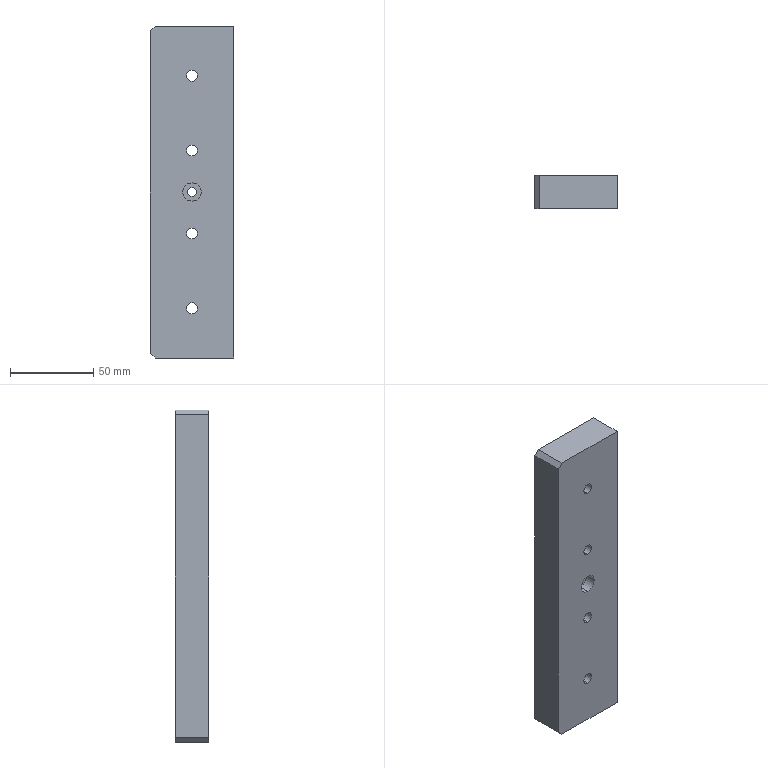Part | SolidWorks | features HoleWzd 3, Chamfer 1, Extrusion 1 | 1 solid | 45 faces | box 50 x 20 x 200 mm | volume 193251 mm3 | cylinder 26 | plane 13 | cone 6 | commonest cylinder face diameters 11 x10 5.2 x8 6.6 x8
STEP:
#1=CARTESIAN_POINT('',(0.,-3.6,5.5));
#2=VERTEX_POINT('',#1);
#3=CARTESIAN_POINT('',(0.,-3.6,-5.5));
#4=VERTEX_POINT('',#3);
#5=CARTESIAN_POINT('',(0.,-3.6,0.));
#6=DIRECTION('',(0.,-1.,0.));
#7=DIRECTION('',(0.,0.,-1.));
#8=AXIS2_PLACEMENT_3D('',#5,#6,#7);
#9=CIRCLE('',#8,5.5);
#10=EDGE_CURVE('',#2,#4,#9,.T.);
#11=ORIENTED_EDGE('',*,*,#10,.F.);
#12=CARTESIAN_POINT('',(0.,-10.,5.5));
#13=VERTEX_POINT('',#12);
#14=CARTESIAN_POINT('',(0.,-10.,5.5));
#15=DIRECTION('',(0.,-1.,0.));
#16=VECTOR('',#15,1000.);
#17=LINE('',#14,#16);
#18=EDGE_CURVE('',#2,#13,#17,.T.);
#19=ORIENTED_EDGE('',*,*,#18,.T.);
#20=CARTESIAN_POINT('',(0.,-10.,-5.5));
#21=VERTEX_POINT('',#20);
#22=CARTESIAN_POINT('',(0.,-10.,0.));
#23=DIRECTION('',(0.,-1.,0.));
#24=DIRECTION('',(0.,0.,-1.));
#25=AXIS2_PLACEMENT_3D('',#22,#23,#24);
#26=CIRCLE('',#25,5.5);
#27=EDGE_CURVE('',#13,#21,#26,.T.);
#28=ORIENTED_EDGE('',*,*,#27,.T.);
#29=CARTESIAN_POINT('',(0.,-10.,-5.5));
#30=DIRECTION('',(0.,-1.,0.));
#31=VECTOR('',#30,1000.);
#32=LINE('',#29,#31);
#33=EDGE_CURVE('',#4,#21,#32,.T.);
#34=ORIENTED_EDGE('',*,*,#33,.F.);
#35=EDGE_LOOP('',(#11,#19,#28,#34));
#36=FACE_OUTER_BOUND('',#35,.T.);
#37=CARTESIAN_POINT('',(0.,-10.,0.));
#38=DIRECTION('',(0.,-1.,0.));
#39=DIRECTION('',(0.,0.,-1.));
#40=AXIS2_PLACEMENT_3D('',#37,#38,#39);
#41=CYLINDRICAL_SURFACE('',#40,5.5);
#42=ADVANCED_FACE('',(#36),#41,.F.);
#43=CARTESIAN_POINT('',(0.,10.,2.6));
#44=VERTEX_POINT('',#43);
#45=CARTESIAN_POINT('',(0.,10.,-2.6));
#46=VERTEX_POINT('',#45);
#47=CARTESIAN_POINT('',(0.,10.,0.));
#48=DIRECTION('',(0.,-1.,0.));
#49=DIRECTION('',(0.,0.,-1.));
#50=AXIS2_PLACEMENT_3D('',#47,#48,#49);
#51=CIRCLE('',#50,2.6);
#52=EDGE_CURVE('',#44,#46,#51,.T.);
#53=ORIENTED_EDGE('',*,*,#52,.F.);
#54=CARTESIAN_POINT('',(0.,-3.6,2.6));
#55=VERTEX_POINT('',#54);
#56=CARTESIAN_POINT('',(0.,-10.,2.6));
#57=DIRECTION('',(0.,-1.,0.));
#58=VECTOR('',#57,1000.);
#59=LINE('',#56,#58);
#60=EDGE_CURVE('',#44,#55,#59,.T.);
#61=ORIENTED_EDGE('',*,*,#60,.T.);
#62=CARTESIAN_POINT('',(0.,-3.6,-2.6));
#63=VERTEX_POINT('',#62);
#64=CARTESIAN_POINT('',(0.,-3.6,0.));
#65=DIRECTION('',(0.,-1.,0.));
#66=DIRECTION('',(0.,0.,-1.));
#67=AXIS2_PLACEMENT_3D('',#64,#65,#66);
#68=CIRCLE('',#67,2.6);
#69=EDGE_CURVE('',#55,#63,#68,.T.);
#70=ORIENTED_EDGE('',*,*,#69,.T.);
#71=CARTESIAN_POINT('',(0.,-10.,-2.6));
#72=DIRECTION('',(0.,-1.,0.));
#73=VECTOR('',#72,1000.);
#74=LINE('',#71,#73);
#75=EDGE_CURVE('',#46,#63,#74,.T.);
#76=ORIENTED_EDGE('',*,*,#75,.F.);
#77=EDGE_LOOP('',(#53,#61,#70,#76));
#78=FACE_OUTER_BOUND('',#77,.T.);
#79=CARTESIAN_POINT('',(0.,-10.,0.));
#80=DIRECTION('',(0.,-1.,0.));
#81=DIRECTION('',(0.,0.,-1.));
#82=AXIS2_PLACEMENT_3D('',#79,#80,#81);
#83=CYLINDRICAL_SURFACE('',#82,2.6);
#84=ADVANCED_FACE('',(#78),#83,.F.);
#85=CARTESIAN_POINT('',(10.,0.,87.6));
#86=VERTEX_POINT('',#85);
#87=CARTESIAN_POINT('',(10.,0.,82.4));
#88=VERTEX_POINT('',#87);
#89=CARTESIAN_POINT('',(10.,0.,85.));
#90=DIRECTION('',(1.,0.,0.));
#91=DIRECTION('',(0.,0.,-1.));
#92=AXIS2_PLACEMENT_3D('',#89,#90,#91);
#93=CIRCLE('',#92,2.6);
#94=EDGE_CURVE('',#86,#88,#93,.T.);
#95=ORIENTED_EDGE('',*,*,#94,.F.);
#96=CARTESIAN_POINT('',(25.,0.,87.6));
#97=VERTEX_POINT('',#96);
#98=CARTESIAN_POINT('',(25.,0.,87.6));
#99=DIRECTION('',(1.,0.,0.));
#100=VECTOR('',#99,1000.);
#101=LINE('',#98,#100);
#102=EDGE_CURVE('',#86,#97,#101,.T.);
#103=ORIENTED_EDGE('',*,*,#102,.T.);
#104=CARTESIAN_POINT('',(25.,0.,82.4));
#105=VERTEX_POINT('',#104);
#106=CARTESIAN_POINT('',(25.,0.,85.));
#107=DIRECTION('',(1.,0.,0.));
#108=DIRECTION('',(0.,0.,-1.));
#109=AXIS2_PLACEMENT_3D('',#106,#107,#108);
#110=CIRCLE('',#109,2.6);
#111=EDGE_CURVE('',#97,#105,#110,.T.);
#112=ORIENTED_EDGE('',*,*,#111,.T.);
#113=CARTESIAN_POINT('',(25.,0.,82.4));
#114=DIRECTION('',(1.,0.,0.));
#115=VECTOR('',#114,1000.);
#116=LINE('',#113,#115);
#117=EDGE_CURVE('',#88,#105,#116,.T.);
#118=ORIENTED_EDGE('',*,*,#117,.F.);
#119=EDGE_LOOP('',(#95,#103,#112,#118));
#120=FACE_OUTER_BOUND('',#119,.T.);
#121=CARTESIAN_POINT('',(25.,0.,85.));
#122=DIRECTION('',(1.,0.,0.));
#123=DIRECTION('',(0.,0.,-1.));
#124=AXIS2_PLACEMENT_3D('',#121,#122,#123);
#125=CYLINDRICAL_SURFACE('',#124,2.6);
#126=ADVANCED_FACE('',(#120),#125,.F.);
#127=CARTESIAN_POINT('',(8.438,0.,85.));
#128=VERTEX_POINT('',#127);
#129=CARTESIAN_POINT('',(10.,0.,82.4));
#130=DIRECTION('',(0.515,0.,-0.8572));
#131=VECTOR('',#130,1000.);
#132=LINE('',#129,#131);
#133=EDGE_CURVE('',#128,#88,#132,.T.);
#134=ORIENTED_EDGE('',*,*,#133,.F.);
#135=CARTESIAN_POINT('',(10.,0.,87.6));
#136=DIRECTION('',(0.515,0.,0.8572));
#137=VECTOR('',#136,1000.);
#138=LINE('',#135,#137);
#139=EDGE_CURVE('',#128,#86,#138,.T.);
#140=ORIENTED_EDGE('',*,*,#139,.T.);
#141=ORIENTED_EDGE('',*,*,#94,.T.);
#142=EDGE_LOOP('',(#134,#140,#141));
#143=FACE_OUTER_BOUND('',#142,.T.);
#144=CARTESIAN_POINT('',(10.,0.,85.));
#145=DIRECTION('',(1.,0.,0.));
#146=DIRECTION('',(0.,0.,-1.));
#147=AXIS2_PLACEMENT_3D('',#144,#145,#146);
#148=CONICAL_SURFACE('',#147,2.6,1.03);
#149=ADVANCED_FACE('',(#143),#148,.F.);
#150=CARTESIAN_POINT('',(10.,0.,2.6));
#151=VERTEX_POINT('',#150);
#152=CARTESIAN_POINT('',(10.,0.,-2.6));
#153=VERTEX_POINT('',#152);
#154=CARTESIAN_POINT('',(10.,0.,0.));
#155=DIRECTION('',(1.,0.,0.));
#156=DIRECTION('',(0.,0.,-1.));
#157=AXIS2_PLACEMENT_3D('',#154,#155,#156);
#158=CIRCLE('',#157,2.6);
#159=EDGE_CURVE('',#151,#153,#158,.T.);
#160=ORIENTED_EDGE('',*,*,#159,.F.);
#161=CARTESIAN_POINT('',(25.,0.,2.6));
#162=VERTEX_POINT('',#161);
#163=CARTESIAN_POINT('',(25.,0.,2.6));
#164=DIRECTION('',(1.,0.,0.));
#165=VECTOR('',#164,1000.);
#166=LINE('',#163,#165);
#167=EDGE_CURVE('',#151,#162,#166,.T.);
#168=ORIENTED_EDGE('',*,*,#167,.T.);
#169=CARTESIAN_POINT('',(25.,0.,-2.6));
#170=VERTEX_POINT('',#169);
#171=CARTESIAN_POINT('',(25.,0.,0.));
#172=DIRECTION('',(1.,0.,0.));
#173=DIRECTION('',(0.,0.,-1.));
#174=AXIS2_PLACEMENT_3D('',#171,#172,#173);
#175=CIRCLE('',#174,2.6);
#176=EDGE_CURVE('',#162,#170,#175,.T.);
#177=ORIENTED_EDGE('',*,*,#176,.T.);
#178=CARTESIAN_POINT('',(25.,0.,-2.6));
#179=DIRECTION('',(1.,0.,0.));
#180=VECTOR('',#179,1000.);
#181=LINE('',#178,#180);
#182=EDGE_CURVE('',#153,#170,#181,.T.);
#183=ORIENTED_EDGE('',*,*,#182,.F.);
#184=EDGE_LOOP('',(#160,#168,#177,#183));
#185=FACE_OUTER_BOUND('',#184,.T.);
#186=CARTESIAN_POINT('',(25.,0.,0.));
#187=DIRECTION('',(1.,0.,0.));
#188=DIRECTION('',(0.,0.,-1.));
#189=AXIS2_PLACEMENT_3D('',#186,#187,#188);
#190=CYLINDRICAL_SURFACE('',#189,2.6);
#191=ADVANCED_FACE('',(#185),#190,.F.);
#192=CARTESIAN_POINT('',(8.438,0.,0.));
#193=VERTEX_POINT('',#192);
#194=CARTESIAN_POINT('',(10.,0.,-2.6));
#195=DIRECTION('',(0.515,0.,-0.8572));
#196=VECTOR('',#195,1000.);
#197=LINE('',#194,#196);
#198=EDGE_CURVE('',#193,#153,#197,.T.);
#199=ORIENTED_EDGE('',*,*,#198,.F.);
#200=CARTESIAN_POINT('',(10.,0.,2.6));
#201=DIRECTION('',(0.515,0.,0.8572));
#202=VECTOR('',#201,1000.);
#203=LINE('',#200,#202);
#204=EDGE_CURVE('',#193,#151,#203,.T.);
#205=ORIENTED_EDGE('',*,*,#204,.T.);
#206=ORIENTED_EDGE('',*,*,#159,.T.);
#207=EDGE_LOOP('',(#199,#205,#206));
#208=FACE_OUTER_BOUND('',#207,.T.);
#209=CARTESIAN_POINT('',(10.,0.,0.));
#210=DIRECTION('',(1.,0.,0.));
#211=DIRECTION('',(0.,0.,-1.));
#212=AXIS2_PLACEMENT_3D('',#209,#210,#211);
#213=CONICAL_SURFACE('',#212,2.6,1.03);
#214=ADVANCED_FACE('',(#208),#213,.F.);
#215=CARTESIAN_POINT('',(10.,0.,-82.4));
#216=VERTEX_POINT('',#215);
#217=CARTESIAN_POINT('',(10.,0.,-87.6));
#218=VERTEX_POINT('',#217);
#219=CARTESIAN_POINT('',(10.,0.,-85.));
#220=DIRECTION('',(1.,0.,0.));
#221=DIRECTION('',(0.,0.,-1.));
#222=AXIS2_PLACEMENT_3D('',#219,#220,#221);
#223=CIRCLE('',#222,2.6);
#224=EDGE_CURVE('',#216,#218,#223,.T.);
#225=ORIENTED_EDGE('',*,*,#224,.F.);
#226=CARTESIAN_POINT('',(25.,0.,-82.4));
#227=VERTEX_POINT('',#226);
#228=CARTESIAN_POINT('',(25.,0.,-82.4));
#229=DIRECTION('',(1.,0.,0.));
#230=VECTOR('',#229,1000.);
#231=LINE('',#228,#230);
#232=EDGE_CURVE('',#216,#227,#231,.T.);
#233=ORIENTED_EDGE('',*,*,#232,.T.);
#234=CARTESIAN_POINT('',(25.,0.,-87.6));
#235=VERTEX_POINT('',#234);
#236=CARTESIAN_POINT('',(25.,0.,-85.));
#237=DIRECTION('',(1.,0.,0.));
#238=DIRECTION('',(0.,0.,-1.));
#239=AXIS2_PLACEMENT_3D('',#236,#237,#238);
#240=CIRCLE('',#239,2.6);
#241=EDGE_CURVE('',#227,#235,#240,.T.);
#242=ORIENTED_EDGE('',*,*,#241,.T.);
#243=CARTESIAN_POINT('',(25.,0.,-87.6));
#244=DIRECTION('',(1.,0.,0.));
#245=VECTOR('',#244,1000.);
#246=LINE('',#243,#245);
#247=EDGE_CURVE('',#218,#235,#246,.T.);
#248=ORIENTED_EDGE('',*,*,#247,.F.);
#249=EDGE_LOOP('',(#225,#233,#242,#248));
#250=FACE_OUTER_BOUND('',#249,.T.);
#251=CARTESIAN_POINT('',(25.,0.,-85.));
#252=DIRECTION('',(1.,0.,0.));
#253=DIRECTION('',(0.,0.,-1.));
#254=AXIS2_PLACEMENT_3D('',#251,#252,#253);
#255=CYLINDRICAL_SURFACE('',#254,2.6);
#256=ADVANCED_FACE('',(#250),#255,.F.);
#257=CARTESIAN_POINT('',(8.438,0.,-85.));
#258=VERTEX_POINT('',#257);
#259=CARTESIAN_POINT('',(10.,0.,-87.6));
#260=DIRECTION('',(0.515,0.,-0.8572));
#261=VECTOR('',#260,1000.);
#262=LINE('',#259,#261);
#263=EDGE_CURVE('',#258,#218,#262,.T.);
#264=ORIENTED_EDGE('',*,*,#263,.F.);
#265=CARTESIAN_POINT('',(10.,0.,-82.4));
#266=DIRECTION('',(0.515,0.,0.8572));
#267=VECTOR('',#266,1000.);
#268=LINE('',#265,#267);
#269=EDGE_CURVE('',#258,#216,#268,.T.);
#270=ORIENTED_EDGE('',*,*,#269,.T.);
#271=ORIENTED_EDGE('',*,*,#224,.T.);
#272=EDGE_LOOP('',(#264,#270,#271));
#273=FACE_OUTER_BOUND('',#272,.T.);
#274=CARTESIAN_POINT('',(10.,0.,-85.));
#275=DIRECTION('',(1.,0.,0.));
#276=DIRECTION('',(0.,0.,-1.));
#277=AXIS2_PLACEMENT_3D('',#274,#275,#276);
#278=CONICAL_SURFACE('',#277,2.6,1.03);
#279=ADVANCED_FACE('',(#273),#278,.F.);
#280=CARTESIAN_POINT('',(0.,2.,-75.5));
#281=VERTEX_POINT('',#280);
#282=CARTESIAN_POINT('',(0.,2.,-64.5));
#283=VERTEX_POINT('',#282);
#284=CARTESIAN_POINT('',(0.,2.,-70.));
#285=DIRECTION('',(0.,1.,0.));
#286=DIRECTION('',(0.,0.,1.));
#287=AXIS2_PLACEMENT_3D('',#284,#285,#286);
#288=CIRCLE('',#287,5.5);
#289=EDGE_CURVE('',#281,#283,#288,.T.);
#290=ORIENTED_EDGE('',*,*,#289,.F.);
#291=CARTESIAN_POINT('',(0.,10.,-75.5));
#292=VERTEX_POINT('',#291);
#293=CARTESIAN_POINT('',(0.,10.,-75.5));
#294=DIRECTION('',(0.,1.,0.));
#295=VECTOR('',#294,1000.);
#296=LINE('',#293,#295);
#297=EDGE_CURVE('',#281,#292,#296,.T.);
#298=ORIENTED_EDGE('',*,*,#297,.T.);
#299=CARTESIAN_POINT('',(0.,10.,-64.5));
#300=VERTEX_POINT('',#299);
#301=CARTESIAN_POINT('',(0.,10.,-70.));
#302=DIRECTION('',(0.,1.,0.));
#303=DIRECTION('',(0.,0.,1.));
#304=AXIS2_PLACEMENT_3D('',#301,#302,#303);
#305=CIRCLE('',#304,5.5);
#306=EDGE_CURVE('',#292,#300,#305,.T.);
#307=ORIENTED_EDGE('',*,*,#306,.T.);
#308=CARTESIAN_POINT('',(0.,10.,-64.5));
#309=DIRECTION('',(0.,1.,0.));
#310=VECTOR('',#309,1000.);
#311=LINE('',#308,#310);
#312=EDGE_CURVE('',#283,#300,#311,.T.);
#313=ORIENTED_EDGE('',*,*,#312,.F.);
#314=EDGE_LOOP('',(#290,#298,#307,#313));
#315=FACE_OUTER_BOUND('',#314,.T.);
#316=CARTESIAN_POINT('',(0.,10.,-70.));
#317=DIRECTION('',(0.,1.,0.));
#318=DIRECTION('',(0.,0.,1.));
#319=AXIS2_PLACEMENT_3D('',#316,#317,#318);
#320=CYLINDRICAL_SURFACE('',#319,5.5);
#321=ADVANCED_FACE('',(#315),#320,.F.);
#322=CARTESIAN_POINT('',(0.,-10.,-73.3));
#323=VERTEX_POINT('',#322);
#324=CARTESIAN_POINT('',(0.,-10.,-66.7));
#325=VERTEX_POINT('',#324);
#326=CARTESIAN_POINT('',(0.,-10.,-70.));
#327=DIRECTION('',(0.,1.,0.));
#328=DIRECTION('',(0.,0.,1.));
#329=AXIS2_PLACEMENT_3D('',#326,#327,#328);
#330=CIRCLE('',#329,3.3);
#331=EDGE_CURVE('',#323,#325,#330,.T.);
#332=ORIENTED_EDGE('',*,*,#331,.F.);
#333=CARTESIAN_POINT('',(0.,2.,-73.3));
#334=VERTEX_POINT('',#333);
#335=CARTESIAN_POINT('',(0.,10.,-73.3));
#336=DIRECTION('',(0.,1.,0.));
#337=VECTOR('',#336,1000.);
#338=LINE('',#335,#337);
#339=EDGE_CURVE('',#323,#334,#338,.T.);
#340=ORIENTED_EDGE('',*,*,#339,.T.);
#341=CARTESIAN_POINT('',(0.,2.,-66.7));
#342=VERTEX_POINT('',#341);
#343=CARTESIAN_POINT('',(0.,2.,-70.));
#344=DIRECTION('',(0.,1.,0.));
#345=DIRECTION('',(0.,0.,1.));
#346=AXIS2_PLACEMENT_3D('',#343,#344,#345);
#347=CIRCLE('',#346,3.3);
#348=EDGE_CURVE('',#334,#342,#347,.T.);
#349=ORIENTED_EDGE('',*,*,#348,.T.);
#350=CARTESIAN_POINT('',(0.,10.,-66.7));
#351=DIRECTION('',(0.,1.,0.));
#352=VECTOR('',#351,1000.);
#353=LINE('',#350,#352);
#354=EDGE_CURVE('',#325,#342,#353,.T.);
#355=ORIENTED_EDGE('',*,*,#354,.F.);
#356=EDGE_LOOP('',(#332,#340,#349,#355));
#357=FACE_OUTER_BOUND('',#356,.T.);
#358=CARTESIAN_POINT('',(0.,10.,-70.));
#359=DIRECTION('',(0.,1.,0.));
#360=DIRECTION('',(0.,0.,1.));
#361=AXIS2_PLACEMENT_3D('',#358,#359,#360);
#362=CYLINDRICAL_SURFACE('',#361,3.3);
#363=ADVANCED_FACE('',(#357),#362,.F.);
#364=CARTESIAN_POINT('',(0.,2.,64.5));
#365=VERTEX_POINT('',#364);
#366=CARTESIAN_POINT('',(0.,2.,75.5));
#367=VERTEX_POINT('',#366);
#368=CARTESIAN_POINT('',(0.,2.,70.));
#369=DIRECTION('',(0.,1.,0.));
#370=DIRECTION('',(0.,0.,1.));
#371=AXIS2_PLACEMENT_3D('',#368,#369,#370);
#372=CIRCLE('',#371,5.5);
#373=EDGE_CURVE('',#365,#367,#372,.T.);
#374=ORIENTED_EDGE('',*,*,#373,.F.);
#375=CARTESIAN_POINT('',(0.,10.,64.5));
#376=VERTEX_POINT('',#375);
#377=CARTESIAN_POINT('',(0.,10.,64.5));
#378=DIRECTION('',(0.,1.,0.));
#379=VECTOR('',#378,1000.);
#380=LINE('',#377,#379);
#381=EDGE_CURVE('',#365,#376,#380,.T.);
#382=ORIENTED_EDGE('',*,*,#381,.T.);
#383=CARTESIAN_POINT('',(0.,10.,75.5));
#384=VERTEX_POINT('',#383);
#385=CARTESIAN_POINT('',(0.,10.,70.));
#386=DIRECTION('',(0.,1.,0.));
#387=DIRECTION('',(0.,0.,1.));
#388=AXIS2_PLACEMENT_3D('',#385,#386,#387);
#389=CIRCLE('',#388,5.5);
#390=EDGE_CURVE('',#376,#384,#389,.T.);
#391=ORIENTED_EDGE('',*,*,#390,.T.);
#392=CARTESIAN_POINT('',(0.,10.,75.5));
#393=DIRECTION('',(0.,1.,0.));
#394=VECTOR('',#393,1000.);
#395=LINE('',#392,#394);
#396=EDGE_CURVE('',#367,#384,#395,.T.);
#397=ORIENTED_EDGE('',*,*,#396,.F.);
#398=EDGE_LOOP('',(#374,#382,#391,#397));
#399=FACE_OUTER_BOUND('',#398,.T.);
#400=CARTESIAN_POINT('',(0.,10.,70.));
#401=DIRECTION('',(0.,1.,0.));
#402=DIRECTION('',(0.,0.,1.));
#403=AXIS2_PLACEMENT_3D('',#400,#401,#402);
#404=CYLINDRICAL_SURFACE('',#403,5.5);
#405=ADVANCED_FACE('',(#399),#404,.F.);
#406=CARTESIAN_POINT('',(0.,-10.,66.7));
#407=VERTEX_POINT('',#406);
#408=CARTESIAN_POINT('',(0.,-10.,73.3));
#409=VERTEX_POINT('',#408);
#410=CARTESIAN_POINT('',(0.,-10.,70.));
#411=DIRECTION('',(0.,1.,0.));
#412=DIRECTION('',(0.,0.,1.));
#413=AXIS2_PLACEMENT_3D('',#410,#411,#412);
#414=CIRCLE('',#413,3.3);
#415=EDGE_CURVE('',#407,#409,#414,.T.);
#416=ORIENTED_EDGE('',*,*,#415,.F.);
#417=CARTESIAN_POINT('',(0.,2.,66.7));
#418=VERTEX_POINT('',#417);
#419=CARTESIAN_POINT('',(0.,10.,66.7));
#420=DIRECTION('',(0.,1.,0.));
#421=VECTOR('',#420,1000.);
#422=LINE('',#419,#421);
#423=EDGE_CURVE('',#407,#418,#422,.T.);
#424=ORIENTED_EDGE('',*,*,#423,.T.);
#425=CARTESIAN_POINT('',(0.,2.,73.3));
#426=VERTEX_POINT('',#425);
#427=CARTESIAN_POINT('',(0.,2.,70.));
#428=DIRECTION('',(0.,1.,0.));
#429=DIRECTION('',(0.,0.,1.));
#430=AXIS2_PLACEMENT_3D('',#427,#428,#429);
#431=CIRCLE('',#430,3.3);
#432=EDGE_CURVE('',#418,#426,#431,.T.);
#433=ORIENTED_EDGE('',*,*,#432,.T.);
#434=CARTESIAN_POINT('',(0.,10.,73.3));
#435=DIRECTION('',(0.,1.,0.));
#436=VECTOR('',#435,1000.);
#437=LINE('',#434,#436);
#438=EDGE_CURVE('',#409,#426,#437,.T.);
#439=ORIENTED_EDGE('',*,*,#438,.F.);
#440=EDGE_LOOP('',(#416,#424,#433,#439));
#441=FACE_OUTER_BOUND('',#440,.T.);
#442=CARTESIAN_POINT('',(0.,10.,70.));
#443=DIRECTION('',(0.,1.,0.));
#444=DIRECTION('',(0.,0.,1.));
#445=AXIS2_PLACEMENT_3D('',#442,#443,#444);
#446=CYLINDRICAL_SURFACE('',#445,3.3);
#447=ADVANCED_FACE('',(#441),#446,.F.);
#448=CARTESIAN_POINT('',(0.,2.,-30.5));
#449=VERTEX_POINT('',#448);
#450=CARTESIAN_POINT('',(0.,2.,-19.5));
#451=VERTEX_POINT('',#450);
#452=CARTESIAN_POINT('',(0.,2.,-25.));
#453=DIRECTION('',(0.,1.,0.));
#454=DIRECTION('',(0.,0.,1.));
#455=AXIS2_PLACEMENT_3D('',#452,#453,#454);
#456=CIRCLE('',#455,5.5);
#457=EDGE_CURVE('',#449,#451,#456,.T.);
#458=ORIENTED_EDGE('',*,*,#457,.F.);
#459=CARTESIAN_POINT('',(0.,10.,-30.5));
#460=VERTEX_POINT('',#459);
#461=CARTESIAN_POINT('',(0.,10.,-30.5));
#462=DIRECTION('',(0.,1.,0.));
#463=VECTOR('',#462,1000.);
#464=LINE('',#461,#463);
#465=EDGE_CURVE('',#449,#460,#464,.T.);
#466=ORIENTED_EDGE('',*,*,#465,.T.);
#467=CARTESIAN_POINT('',(0.,10.,-19.5));
#468=VERTEX_POINT('',#467);
#469=CARTESIAN_POINT('',(0.,10.,-25.));
#470=DIRECTION('',(0.,1.,0.));
#471=DIRECTION('',(0.,0.,1.));
#472=AXIS2_PLACEMENT_3D('',#469,#470,#471);
#473=CIRCLE('',#472,5.5);
#474=EDGE_CURVE('',#460,#468,#473,.T.);
#475=ORIENTED_EDGE('',*,*,#474,.T.);
#476=CARTESIAN_POINT('',(0.,10.,-19.5));
#477=DIRECTION('',(0.,1.,0.));
#478=VECTOR('',#477,1000.);
#479=LINE('',#476,#478);
#480=EDGE_CURVE('',#451,#468,#479,.T.);
#481=ORIENTED_EDGE('',*,*,#480,.F.);
#482=EDGE_LOOP('',(#458,#466,#475,#481));
#483=FACE_OUTER_BOUND('',#482,.T.);
#484=CARTESIAN_POINT('',(0.,10.,-25.));
#485=DIRECTION('',(0.,1.,0.));
#486=DIRECTION('',(0.,0.,1.));
#487=AXIS2_PLACEMENT_3D('',#484,#485,#486);
#488=CYLINDRICAL_SURFACE('',#487,5.5);
#489=ADVANCED_FACE('',(#483),#488,.F.);
#490=CARTESIAN_POINT('',(0.,-10.,-28.3));
#491=VERTEX_POINT('',#490);
#492=CARTESIAN_POINT('',(0.,-10.,-21.7));
#493=VERTEX_POINT('',#492);
#494=CARTESIAN_POINT('',(0.,-10.,-25.));
#495=DIRECTION('',(0.,1.,0.));
#496=DIRECTION('',(0.,0.,1.));
#497=AXIS2_PLACEMENT_3D('',#494,#495,#496);
#498=CIRCLE('',#497,3.3);
#499=EDGE_CURVE('',#491,#493,#498,.T.);
#500=ORIENTED_EDGE('',*,*,#499,.F.);
#501=CARTESIAN_POINT('',(0.,2.,-28.3));
#502=VERTEX_POINT('',#501);
#503=CARTESIAN_POINT('',(0.,10.,-28.3));
#504=DIRECTION('',(0.,1.,0.));
#505=VECTOR('',#504,1000.);
#506=LINE('',#503,#505);
#507=EDGE_CURVE('',#491,#502,#506,.T.);
#508=ORIENTED_EDGE('',*,*,#507,.T.);
#509=CARTESIAN_POINT('',(0.,2.,-21.7));
#510=VERTEX_POINT('',#509);
#511=CARTESIAN_POINT('',(0.,2.,-25.));
#512=DIRECTION('',(0.,1.,0.));
#513=DIRECTION('',(0.,0.,1.));
#514=AXIS2_PLACEMENT_3D('',#511,#512,#513);
#515=CIRCLE('',#514,3.3);
#516=EDGE_CURVE('',#502,#510,#515,.T.);
#517=ORIENTED_EDGE('',*,*,#516,.T.);
#518=CARTESIAN_POINT('',(0.,10.,-21.7));
#519=DIRECTION('',(0.,1.,0.));
#520=VECTOR('',#519,1000.);
#521=LINE('',#518,#520);
#522=EDGE_CURVE('',#493,#510,#521,.T.);
#523=ORIENTED_EDGE('',*,*,#522,.F.);
#524=EDGE_LOOP('',(#500,#508,#517,#523));
#525=FACE_OUTER_BOUND('',#524,.T.);
#526=CARTESIAN_POINT('',(0.,10.,-25.));
#527=DIRECTION('',(0.,1.,0.));
#528=DIRECTION('',(0.,0.,1.));
#529=AXIS2_PLACEMENT_3D('',#526,#527,#528);
#530=CYLINDRICAL_SURFACE('',#529,3.3);
#531=ADVANCED_FACE('',(#525),#530,.F.);
#532=CARTESIAN_POINT('',(0.,2.,19.5));
#533=VERTEX_POINT('',#532);
#534=CARTESIAN_POINT('',(0.,2.,30.5));
#535=VERTEX_POINT('',#534);
#536=CARTESIAN_POINT('',(0.,2.,25.));
#537=DIRECTION('',(0.,1.,0.));
#538=DIRECTION('',(0.,0.,1.));
#539=AXIS2_PLACEMENT_3D('',#536,#537,#538);
#540=CIRCLE('',#539,5.5);
#541=EDGE_CURVE('',#533,#535,#540,.T.);
#542=ORIENTED_EDGE('',*,*,#541,.F.);
#543=CARTESIAN_POINT('',(0.,10.,19.5));
#544=VERTEX_POINT('',#543);
#545=CARTESIAN_POINT('',(0.,10.,19.5));
#546=DIRECTION('',(0.,1.,0.));
#547=VECTOR('',#546,1000.);
#548=LINE('',#545,#547);
#549=EDGE_CURVE('',#533,#544,#548,.T.);
#550=ORIENTED_EDGE('',*,*,#549,.T.);
#551=CARTESIAN_POINT('',(0.,10.,30.5));
#552=VERTEX_POINT('',#551);
#553=CARTESIAN_POINT('',(0.,10.,25.));
#554=DIRECTION('',(0.,1.,0.));
#555=DIRECTION('',(0.,0.,1.));
#556=AXIS2_PLACEMENT_3D('',#553,#554,#555);
#557=CIRCLE('',#556,5.5);
#558=EDGE_CURVE('',#544,#552,#557,.T.);
#559=ORIENTED_EDGE('',*,*,#558,.T.);
#560=CARTESIAN_POINT('',(0.,10.,30.5));
#561=DIRECTION('',(0.,1.,0.));
#562=VECTOR('',#561,1000.);
#563=LINE('',#560,#562);
#564=EDGE_CURVE('',#535,#552,#563,.T.);
#565=ORIENTED_EDGE('',*,*,#564,.F.);
#566=EDGE_LOOP('',(#542,#550,#559,#565));
#567=FACE_OUTER_BOUND('',#566,.T.);
#568=CARTESIAN_POINT('',(0.,10.,25.));
#569=DIRECTION('',(0.,1.,0.));
#570=DIRECTION('',(0.,0.,1.));
#571=AXIS2_PLACEMENT_3D('',#568,#569,#570);
#572=CYLINDRICAL_SURFACE('',#571,5.5);
#573=ADVANCED_FACE('',(#567),#572,.F.);
#574=CARTESIAN_POINT('',(0.,-10.,21.7));
#575=VERTEX_POINT('',#574);
#576=CARTESIAN_POINT('',(0.,-10.,28.3));
#577=VERTEX_POINT('',#576);
#578=CARTESIAN_POINT('',(0.,-10.,25.));
#579=DIRECTION('',(0.,1.,0.));
#580=DIRECTION('',(0.,0.,1.));
#581=AXIS2_PLACEMENT_3D('',#578,#579,#580);
#582=CIRCLE('',#581,3.3);
#583=EDGE_CURVE('',#575,#577,#582,.T.);
#584=ORIENTED_EDGE('',*,*,#583,.F.);
#585=CARTESIAN_POINT('',(0.,2.,21.7));
#586=VERTEX_POINT('',#585);
#587=CARTESIAN_POINT('',(0.,10.,21.7));
#588=DIRECTION('',(0.,1.,0.));
#589=VECTOR('',#588,1000.);
#590=LINE('',#587,#589);
#591=EDGE_CURVE('',#575,#586,#590,.T.);
#592=ORIENTED_EDGE('',*,*,#591,.T.);
#593=CARTESIAN_POINT('',(0.,2.,28.3));
#594=VERTEX_POINT('',#593);
#595=CARTESIAN_POINT('',(0.,2.,25.));
#596=DIRECTION('',(0.,1.,0.));
#597=DIRECTION('',(0.,0.,1.));
#598=AXIS2_PLACEMENT_3D('',#595,#596,#597);
#599=CIRCLE('',#598,3.3);
#600=EDGE_CURVE('',#586,#594,#599,.T.);
#601=ORIENTED_EDGE('',*,*,#600,.T.);
#602=CARTESIAN_POINT('',(0.,10.,28.3));
#603=DIRECTION('',(0.,1.,0.));
#604=VECTOR('',#603,1000.);
#605=LINE('',#602,#604);
#606=EDGE_CURVE('',#577,#594,#605,.T.);
#607=ORIENTED_EDGE('',*,*,#606,.F.);
#608=EDGE_LOOP('',(#584,#592,#601,#607));
#609=FACE_OUTER_BOUND('',#608,.T.);
#610=CARTESIAN_POINT('',(0.,10.,25.));
#611=DIRECTION('',(0.,1.,0.));
#612=DIRECTION('',(0.,0.,1.));
#613=AXIS2_PLACEMENT_3D('',#610,#611,#612);
#614=CYLINDRICAL_SURFACE('',#613,3.3);
#615=ADVANCED_FACE('',(#609),#614,.F.);
#616=CARTESIAN_POINT('',(-25.,-10.,-97.));
#617=VERTEX_POINT('',#616);
#618=CARTESIAN_POINT('',(-25.,-10.,97.));
#619=VERTEX_POINT('',#618);
#620=CARTESIAN_POINT('',(-25.,-10.,100.));
#621=DIRECTION('',(0.,0.,1.));
#622=VECTOR('',#621,1000.);
#623=LINE('',#620,#622);
#624=EDGE_CURVE('',#617,#619,#623,.T.);
#625=ORIENTED_EDGE('',*,*,#624,.T.);
#626=CARTESIAN_POINT('',(-25.,10.,97.));
#627=VERTEX_POINT('',#626);
#628=CARTESIAN_POINT('',(-25.,10.,97.));
#629=DIRECTION('',(0.,1.,0.));
#630=VECTOR('',#629,1000.);
#631=LINE('',#628,#630);
#632=EDGE_CURVE('',#619,#627,#631,.T.);
#633=ORIENTED_EDGE('',*,*,#632,.T.);
#634=CARTESIAN_POINT('',(-25.,10.,-97.));
#635=VERTEX_POINT('',#634);
#636=CARTESIAN_POINT('',(-25.,10.,100.));
#637=DIRECTION('',(0.,0.,1.));
#638=VECTOR('',#637,1000.);
#639=LINE('',#636,#638);
#640=EDGE_CURVE('',#635,#627,#639,.T.);
#641=ORIENTED_EDGE('',*,*,#640,.F.);
#642=CARTESIAN_POINT('',(-25.,10.,-97.));
#643=DIRECTION('',(0.,-1.,0.));
#644=VECTOR('',#643,1000.);
#645=LINE('',#642,#644);
#646=EDGE_CURVE('',#635,#617,#645,.T.);
#647=ORIENTED_EDGE('',*,*,#646,.T.);
#648=EDGE_LOOP('',(#625,#633,#641,#647));
#649=FACE_OUTER_BOUND('',#648,.T.);
#650=CARTESIAN_POINT('',(-25.,10.,100.));
#651=DIRECTION('',(1.,0.,0.));
#652=DIRECTION('',(0.,0.,-1.));
#653=AXIS2_PLACEMENT_3D('',#650,#651,#652);
#654=PLANE('',#653);
#655=ADVANCED_FACE('',(#649),#654,.F.);
#656=CARTESIAN_POINT('',(-22.,10.,100.));
#657=VERTEX_POINT('',#656);
#658=CARTESIAN_POINT('',(25.,10.,100.));
#659=VERTEX_POINT('',#658);
#660=CARTESIAN_POINT('',(25.,10.,100.));
#661=DIRECTION('',(1.,0.,0.));
#662=VECTOR('',#661,1000.);
#663=LINE('',#660,#662);
#664=EDGE_CURVE('',#657,#659,#663,.T.);
#665=ORIENTED_EDGE('',*,*,#664,.F.);
#666=CARTESIAN_POINT('',(-22.,-10.,100.));
#667=VERTEX_POINT('',#666);
#668=CARTESIAN_POINT('',(-22.,10.,100.));
#669=DIRECTION('',(0.,-1.,0.));
#670=VECTOR('',#669,1000.);
#671=LINE('',#668,#670);
#672=EDGE_CURVE('',#657,#667,#671,.T.);
#673=ORIENTED_EDGE('',*,*,#672,.T.);
#674=CARTESIAN_POINT('',(25.,-10.,100.));
#675=VERTEX_POINT('',#674);
#676=CARTESIAN_POINT('',(25.,-10.,100.));
#677=DIRECTION('',(1.,0.,0.));
#678=VECTOR('',#677,1000.);
#679=LINE('',#676,#678);
#680=EDGE_CURVE('',#667,#675,#679,.T.);
#681=ORIENTED_EDGE('',*,*,#680,.T.);
#682=CARTESIAN_POINT('',(25.,10.,100.));
#683=DIRECTION('',(0.,-1.,0.));
#684=VECTOR('',#683,1000.);
#685=LINE('',#682,#684);
#686=EDGE_CURVE('',#659,#675,#685,.T.);
#687=ORIENTED_EDGE('',*,*,#686,.F.);
#688=EDGE_LOOP('',(#665,#673,#681,#687));
#689=FACE_OUTER_BOUND('',#688,.T.);
#690=CARTESIAN_POINT('',(25.,10.,100.));
#691=DIRECTION('',(0.,0.,-1.));
#692=DIRECTION('',(-1.,0.,0.));
#693=AXIS2_PLACEMENT_3D('',#690,#691,#692);
#694=PLANE('',#693);
#695=ADVANCED_FACE('',(#689),#694,.F.);
#696=CARTESIAN_POINT('',(25.,0.,85.));
#697=DIRECTION('',(1.,0.,0.));
#698=DIRECTION('',(0.,0.,-1.));
#699=AXIS2_PLACEMENT_3D('',#696,#697,#698);
#700=CIRCLE('',#699,2.6);
#701=EDGE_CURVE('',#105,#97,#700,.T.);
#702=ORIENTED_EDGE('',*,*,#701,.F.);
#703=ORIENTED_EDGE('',*,*,#111,.F.);
#704=EDGE_LOOP('',(#702,#703));
#705=FACE_BOUND('',#704,.T.);
#706=CARTESIAN_POINT('',(25.,0.,0.));
#707=DIRECTION('',(1.,0.,0.));
#708=DIRECTION('',(0.,0.,-1.));
#709=AXIS2_PLACEMENT_3D('',#706,#707,#708);
#710=CIRCLE('',#709,2.6);
#711=EDGE_CURVE('',#170,#162,#710,.T.);
#712=ORIENTED_EDGE('',*,*,#711,.F.);
#713=ORIENTED_EDGE('',*,*,#176,.F.);
#714=EDGE_LOOP('',(#712,#713));
#715=FACE_BOUND('',#714,.T.);
#716=CARTESIAN_POINT('',(25.,0.,-85.));
#717=DIRECTION('',(1.,0.,0.));
#718=DIRECTION('',(0.,0.,-1.));
#719=AXIS2_PLACEMENT_3D('',#716,#717,#718);
#720=CIRCLE('',#719,2.6);
#721=EDGE_CURVE('',#235,#227,#720,.T.);
#722=ORIENTED_EDGE('',*,*,#721,.F.);
#723=ORIENTED_EDGE('',*,*,#241,.F.);
#724=EDGE_LOOP('',(#722,#723));
#725=FACE_BOUND('',#724,.T.);
#726=CARTESIAN_POINT('',(25.,-10.,-100.));
#727=VERTEX_POINT('',#726);
#728=CARTESIAN_POINT('',(25.,-10.,100.));
#729=DIRECTION('',(0.,0.,-1.));
#730=VECTOR('',#729,1000.);
#731=LINE('',#728,#730);
#732=EDGE_CURVE('',#675,#727,#731,.T.);
#733=ORIENTED_EDGE('',*,*,#732,.T.);
#734=CARTESIAN_POINT('',(25.,10.,-100.));
#735=VERTEX_POINT('',#734);
#736=CARTESIAN_POINT('',(25.,10.,-100.));
#737=DIRECTION('',(0.,-1.,0.));
#738=VECTOR('',#737,1000.);
#739=LINE('',#736,#738);
#740=EDGE_CURVE('',#735,#727,#739,.T.);
#741=ORIENTED_EDGE('',*,*,#740,.F.);
#742=CARTESIAN_POINT('',(25.,10.,100.));
#743=DIRECTION('',(0.,0.,-1.));
#744=VECTOR('',#743,1000.);
#745=LINE('',#742,#744);
#746=EDGE_CURVE('',#659,#735,#745,.T.);
#747=ORIENTED_EDGE('',*,*,#746,.F.);
#748=ORIENTED_EDGE('',*,*,#686,.T.);
#749=EDGE_LOOP('',(#733,#741,#747,#748));
#750=FACE_OUTER_BOUND('',#749,.T.);
#751=CARTESIAN_POINT('',(25.,10.,100.));
#752=DIRECTION('',(-1.,0.,0.));
#753=DIRECTION('',(0.,0.,1.));
#754=AXIS2_PLACEMENT_3D('',#751,#752,#753);
#755=PLANE('',#754);
#756=ADVANCED_FACE('',(#705,#715,#725,#750),#755,.F.);
#757=CARTESIAN_POINT('',(-22.,-10.,-100.));
#758=VERTEX_POINT('',#757);
#759=CARTESIAN_POINT('',(25.,-10.,-100.));
#760=DIRECTION('',(-1.,0.,0.));
#761=VECTOR('',#760,1000.);
#762=LINE('',#759,#761);
#763=EDGE_CURVE('',#727,#758,#762,.T.);
#764=ORIENTED_EDGE('',*,*,#763,.T.);
#765=CARTESIAN_POINT('',(-22.,10.,-100.));
#766=VERTEX_POINT('',#765);
#767=CARTESIAN_POINT('',(-22.,10.,-100.));
#768=DIRECTION('',(0.,1.,0.));
#769=VECTOR('',#768,1000.);
#770=LINE('',#767,#769);
#771=EDGE_CURVE('',#758,#766,#770,.T.);
#772=ORIENTED_EDGE('',*,*,#771,.T.);
#773=CARTESIAN_POINT('',(25.,10.,-100.));
#774=DIRECTION('',(-1.,0.,0.));
#775=VECTOR('',#774,1000.);
#776=LINE('',#773,#775);
#777=EDGE_CURVE('',#735,#766,#776,.T.);
#778=ORIENTED_EDGE('',*,*,#777,.F.);
#779=ORIENTED_EDGE('',*,*,#740,.T.);
#780=EDGE_LOOP('',(#764,#772,#778,#779));
#781=FACE_OUTER_BOUND('',#780,.T.);
#782=CARTESIAN_POINT('',(25.,10.,-100.));
#783=DIRECTION('',(0.,0.,1.));
#784=DIRECTION('',(1.,0.,0.));
#785=AXIS2_PLACEMENT_3D('',#782,#783,#784);
#786=PLANE('',#785);
#787=ADVANCED_FACE('',(#781),#786,.F.);
#788=CARTESIAN_POINT('',(0.,10.,0.));
#789=DIRECTION('',(0.,-1.,0.));
#790=DIRECTION('',(0.,0.,-1.));
#791=AXIS2_PLACEMENT_3D('',#788,#789,#790);
#792=CIRCLE('',#791,2.6);
#793=EDGE_CURVE('',#46,#44,#792,.T.);
#794=ORIENTED_EDGE('',*,*,#793,.T.);
#795=ORIENTED_EDGE('',*,*,#52,.T.);
#796=EDGE_LOOP('',(#794,#795));
#797=FACE_BOUND('',#796,.T.);
#798=CARTESIAN_POINT('',(0.,10.,-70.));
#799=DIRECTION('',(0.,1.,0.));
#800=DIRECTION('',(0.,0.,1.));
#801=AXIS2_PLACEMENT_3D('',#798,#799,#800);
#802=CIRCLE('',#801,5.5);
#803=EDGE_CURVE('',#300,#292,#802,.T.);
#804=ORIENTED_EDGE('',*,*,#803,.F.);
#805=ORIENTED_EDGE('',*,*,#306,.F.);
#806=EDGE_LOOP('',(#804,#805));
#807=FACE_BOUND('',#806,.T.);
#808=CARTESIAN_POINT('',(0.,10.,70.));
#809=DIRECTION('',(0.,1.,0.));
#810=DIRECTION('',(0.,0.,1.));
#811=AXIS2_PLACEMENT_3D('',#808,#809,#810);
#812=CIRCLE('',#811,5.5);
#813=EDGE_CURVE('',#384,#376,#812,.T.);
#814=ORIENTED_EDGE('',*,*,#813,.F.);
#815=ORIENTED_EDGE('',*,*,#390,.F.);
#816=EDGE_LOOP('',(#814,#815));
#817=FACE_BOUND('',#816,.T.);
#818=CARTESIAN_POINT('',(0.,10.,-25.));
#819=DIRECTION('',(0.,1.,0.));
#820=DIRECTION('',(0.,0.,1.));
#821=AXIS2_PLACEMENT_3D('',#818,#819,#820);
#822=CIRCLE('',#821,5.5);
#823=EDGE_CURVE('',#468,#460,#822,.T.);
#824=ORIENTED_EDGE('',*,*,#823,.F.);
#825=ORIENTED_EDGE('',*,*,#474,.F.);
#826=EDGE_LOOP('',(#824,#825));
#827=FACE_BOUND('',#826,.T.);
#828=CARTESIAN_POINT('',(0.,10.,25.));
#829=DIRECTION('',(0.,1.,0.));
#830=DIRECTION('',(0.,0.,1.));
#831=AXIS2_PLACEMENT_3D('',#828,#829,#830);
#832=CIRCLE('',#831,5.5);
#833=EDGE_CURVE('',#552,#544,#832,.T.);
#834=ORIENTED_EDGE('',*,*,#833,.F.);
#835=ORIENTED_EDGE('',*,*,#558,.F.);
#836=EDGE_LOOP('',(#834,#835));
#837=FACE_BOUND('',#836,.T.);
#838=ORIENTED_EDGE('',*,*,#640,.T.);
#839=CARTESIAN_POINT('',(-61.,10.,61.));
#840=DIRECTION('',(0.7071,0.,0.7071));
#841=VECTOR('',#840,1000.);
#842=LINE('',#839,#841);
#843=EDGE_CURVE('',#627,#657,#842,.T.);
#844=ORIENTED_EDGE('',*,*,#843,.T.);
#845=ORIENTED_EDGE('',*,*,#664,.T.);
#846=ORIENTED_EDGE('',*,*,#746,.T.);
#847=ORIENTED_EDGE('',*,*,#777,.T.);
#848=CARTESIAN_POINT('',(-61.,10.,-61.));
#849=DIRECTION('',(-0.7071,0.,0.7071));
#850=VECTOR('',#849,1000.);
#851=LINE('',#848,#850);
#852=EDGE_CURVE('',#766,#635,#851,.T.);
#853=ORIENTED_EDGE('',*,*,#852,.T.);
#854=EDGE_LOOP('',(#838,#844,#845,#846,#847,#853));
#855=FACE_OUTER_BOUND('',#854,.T.);
#856=CARTESIAN_POINT('',(0.,10.,0.));
#857=DIRECTION('',(0.,1.,0.));
#858=DIRECTION('',(0.,0.,1.));
#859=AXIS2_PLACEMENT_3D('',#856,#857,#858);
#860=PLANE('',#859);
#861=ADVANCED_FACE('',(#797,#807,#817,#827,#837,#855),#860,.T.);
#862=CARTESIAN_POINT('',(0.,-10.,0.));
#863=DIRECTION('',(0.,-1.,0.));
#864=DIRECTION('',(0.,0.,-1.));
#865=AXIS2_PLACEMENT_3D('',#862,#863,#864);
#866=CIRCLE('',#865,5.5);
#867=EDGE_CURVE('',#21,#13,#866,.T.);
#868=ORIENTED_EDGE('',*,*,#867,.F.);
#869=ORIENTED_EDGE('',*,*,#27,.F.);
#870=EDGE_LOOP('',(#868,#869));
#871=FACE_BOUND('',#870,.T.);
#872=CARTESIAN_POINT('',(0.,-10.,-70.));
#873=DIRECTION('',(0.,1.,0.));
#874=DIRECTION('',(0.,0.,1.));
#875=AXIS2_PLACEMENT_3D('',#872,#873,#874);
#876=CIRCLE('',#875,3.3);
#877=EDGE_CURVE('',#325,#323,#876,.T.);
#878=ORIENTED_EDGE('',*,*,#877,.T.);
#879=ORIENTED_EDGE('',*,*,#331,.T.);
#880=EDGE_LOOP('',(#878,#879));
#881=FACE_BOUND('',#880,.T.);
#882=CARTESIAN_POINT('',(0.,-10.,70.));
#883=DIRECTION('',(0.,1.,0.));
#884=DIRECTION('',(0.,0.,1.));
#885=AXIS2_PLACEMENT_3D('',#882,#883,#884);
#886=CIRCLE('',#885,3.3);
#887=EDGE_CURVE('',#409,#407,#886,.T.);
#888=ORIENTED_EDGE('',*,*,#887,.T.);
#889=ORIENTED_EDGE('',*,*,#415,.T.);
#890=EDGE_LOOP('',(#888,#889));
#891=FACE_BOUND('',#890,.T.);
#892=CARTESIAN_POINT('',(0.,-10.,-25.));
#893=DIRECTION('',(0.,1.,0.));
#894=DIRECTION('',(0.,0.,1.));
#895=AXIS2_PLACEMENT_3D('',#892,#893,#894);
#896=CIRCLE('',#895,3.3);
#897=EDGE_CURVE('',#493,#491,#896,.T.);
#898=ORIENTED_EDGE('',*,*,#897,.T.);
#899=ORIENTED_EDGE('',*,*,#499,.T.);
#900=EDGE_LOOP('',(#898,#899));
#901=FACE_BOUND('',#900,.T.);
#902=CARTESIAN_POINT('',(0.,-10.,25.));
#903=DIRECTION('',(0.,1.,0.));
#904=DIRECTION('',(0.,0.,1.));
#905=AXIS2_PLACEMENT_3D('',#902,#903,#904);
#906=CIRCLE('',#905,3.3);
#907=EDGE_CURVE('',#577,#575,#906,.T.);
#908=ORIENTED_EDGE('',*,*,#907,.T.);
#909=ORIENTED_EDGE('',*,*,#583,.T.);
#910=EDGE_LOOP('',(#908,#909));
#911=FACE_BOUND('',#910,.T.);
#912=ORIENTED_EDGE('',*,*,#680,.F.);
#913=CARTESIAN_POINT('',(-22.,-10.,100.));
#914=DIRECTION('',(-0.7071,0.,-0.7071));
#915=VECTOR('',#914,1000.);
#916=LINE('',#913,#915);
#917=EDGE_CURVE('',#667,#619,#916,.T.);
#918=ORIENTED_EDGE('',*,*,#917,.T.);
#919=ORIENTED_EDGE('',*,*,#624,.F.);
#920=CARTESIAN_POINT('',(-25.,-10.,-97.));
#921=DIRECTION('',(0.7071,0.,-0.7071));
#922=VECTOR('',#921,1000.);
#923=LINE('',#920,#922);
#924=EDGE_CURVE('',#617,#758,#923,.T.);
#925=ORIENTED_EDGE('',*,*,#924,.T.);
#926=ORIENTED_EDGE('',*,*,#763,.F.);
#927=ORIENTED_EDGE('',*,*,#732,.F.);
#928=EDGE_LOOP('',(#912,#918,#919,#925,#926,#927));
#929=FACE_OUTER_BOUND('',#928,.T.);
#930=CARTESIAN_POINT('',(0.,-10.,0.));
#931=DIRECTION('',(0.,1.,0.));
#932=DIRECTION('',(0.,0.,1.));
#933=AXIS2_PLACEMENT_3D('',#930,#931,#932);
#934=PLANE('',#933);
#935=ADVANCED_FACE('',(#871,#881,#891,#901,#911,#929),#934,.F.);
#936=ORIENTED_EDGE('',*,*,#591,.F.);
#937=ORIENTED_EDGE('',*,*,#907,.F.);
#938=ORIENTED_EDGE('',*,*,#606,.T.);
#939=CARTESIAN_POINT('',(0.,2.,25.));
#940=DIRECTION('',(0.,1.,0.));
#941=DIRECTION('',(0.,0.,1.));
#942=AXIS2_PLACEMENT_3D('',#939,#940,#941);
#943=CIRCLE('',#942,3.3);
#944=EDGE_CURVE('',#594,#586,#943,.T.);
#945=ORIENTED_EDGE('',*,*,#944,.T.);
#946=EDGE_LOOP('',(#936,#937,#938,#945));
#947=FACE_OUTER_BOUND('',#946,.T.);
#948=CARTESIAN_POINT('',(0.,10.,25.));
#949=DIRECTION('',(0.,1.,0.));
#950=DIRECTION('',(0.,0.,1.));
#951=AXIS2_PLACEMENT_3D('',#948,#949,#950);
#952=CYLINDRICAL_SURFACE('',#951,3.3);
#953=ADVANCED_FACE('',(#947),#952,.F.);
#954=ORIENTED_EDGE('',*,*,#944,.F.);
#955=ORIENTED_EDGE('',*,*,#600,.F.);
#956=EDGE_LOOP('',(#954,#955));
#957=FACE_BOUND('',#956,.T.);
#958=CARTESIAN_POINT('',(0.,2.,25.));
#959=DIRECTION('',(0.,1.,0.));
#960=DIRECTION('',(0.,0.,1.));
#961=AXIS2_PLACEMENT_3D('',#958,#959,#960);
#962=CIRCLE('',#961,5.5);
#963=EDGE_CURVE('',#535,#533,#962,.T.);
#964=ORIENTED_EDGE('',*,*,#963,.T.);
#965=ORIENTED_EDGE('',*,*,#541,.T.);
#966=EDGE_LOOP('',(#964,#965));
#967=FACE_OUTER_BOUND('',#966,.T.);
#968=CARTESIAN_POINT('',(3.3,2.,25.));
#969=DIRECTION('',(0.,-1.,0.));
#970=DIRECTION('',(0.,0.,-1.));
#971=AXIS2_PLACEMENT_3D('',#968,#969,#970);
#972=PLANE('',#971);
#973=ADVANCED_FACE('',(#957,#967),#972,.F.);
#974=ORIENTED_EDGE('',*,*,#549,.F.);
#975=ORIENTED_EDGE('',*,*,#963,.F.);
#976=ORIENTED_EDGE('',*,*,#564,.T.);
#977=ORIENTED_EDGE('',*,*,#833,.T.);
#978=EDGE_LOOP('',(#974,#975,#976,#977));
#979=FACE_OUTER_BOUND('',#978,.T.);
#980=CARTESIAN_POINT('',(0.,10.,25.));
#981=DIRECTION('',(0.,1.,0.));
#982=DIRECTION('',(0.,0.,1.));
#983=AXIS2_PLACEMENT_3D('',#980,#981,#982);
#984=CYLINDRICAL_SURFACE('',#983,5.5);
#985=ADVANCED_FACE('',(#979),#984,.F.);
#986=ORIENTED_EDGE('',*,*,#507,.F.);
#987=ORIENTED_EDGE('',*,*,#897,.F.);
#988=ORIENTED_EDGE('',*,*,#522,.T.);
#989=CARTESIAN_POINT('',(0.,2.,-25.));
#990=DIRECTION('',(0.,1.,0.));
#991=DIRECTION('',(0.,0.,1.));
#992=AXIS2_PLACEMENT_3D('',#989,#990,#991);
#993=CIRCLE('',#992,3.3);
#994=EDGE_CURVE('',#510,#502,#993,.T.);
#995=ORIENTED_EDGE('',*,*,#994,.T.);
#996=EDGE_LOOP('',(#986,#987,#988,#995));
#997=FACE_OUTER_BOUND('',#996,.T.);
#998=CARTESIAN_POINT('',(0.,10.,-25.));
#999=DIRECTION('',(0.,1.,0.));
#1000=DIRECTION('',(0.,0.,1.));
#1001=AXIS2_PLACEMENT_3D('',#998,#999,#1000);
#1002=CYLINDRICAL_SURFACE('',#1001,3.3);
#1003=ADVANCED_FACE('',(#997),#1002,.F.);
#1004=ORIENTED_EDGE('',*,*,#994,.F.);
#1005=ORIENTED_EDGE('',*,*,#516,.F.);
#1006=EDGE_LOOP('',(#1004,#1005));
#1007=FACE_BOUND('',#1006,.T.);
#1008=CARTESIAN_POINT('',(0.,2.,-25.));
#1009=DIRECTION('',(0.,1.,0.));
#1010=DIRECTION('',(0.,0.,1.));
#1011=AXIS2_PLACEMENT_3D('',#1008,#1009,#1010);
#1012=CIRCLE('',#1011,5.5);
#1013=EDGE_CURVE('',#451,#449,#1012,.T.);
#1014=ORIENTED_EDGE('',*,*,#1013,.T.);
#1015=ORIENTED_EDGE('',*,*,#457,.T.);
#1016=EDGE_LOOP('',(#1014,#1015));
#1017=FACE_OUTER_BOUND('',#1016,.T.);
#1018=CARTESIAN_POINT('',(3.3,2.,-25.));
#1019=DIRECTION('',(0.,-1.,0.));
#1020=DIRECTION('',(0.,0.,-1.));
#1021=AXIS2_PLACEMENT_3D('',#1018,#1019,#1020);
#1022=PLANE('',#1021);
#1023=ADVANCED_FACE('',(#1007,#1017),#1022,.F.);
#1024=ORIENTED_EDGE('',*,*,#465,.F.);
#1025=ORIENTED_EDGE('',*,*,#1013,.F.);
#1026=ORIENTED_EDGE('',*,*,#480,.T.);
#1027=ORIENTED_EDGE('',*,*,#823,.T.);
#1028=EDGE_LOOP('',(#1024,#1025,#1026,#1027));
#1029=FACE_OUTER_BOUND('',#1028,.T.);
#1030=CARTESIAN_POINT('',(0.,10.,-25.));
#1031=DIRECTION('',(0.,1.,0.));
#1032=DIRECTION('',(0.,0.,1.));
#1033=AXIS2_PLACEMENT_3D('',#1030,#1031,#1032);
#1034=CYLINDRICAL_SURFACE('',#1033,5.5);
#1035=ADVANCED_FACE('',(#1029),#1034,.F.);
#1036=ORIENTED_EDGE('',*,*,#423,.F.);
#1037=ORIENTED_EDGE('',*,*,#887,.F.);
#1038=ORIENTED_EDGE('',*,*,#438,.T.);
#1039=CARTESIAN_POINT('',(0.,2.,70.));
#1040=DIRECTION('',(0.,1.,0.));
#1041=DIRECTION('',(0.,0.,1.));
#1042=AXIS2_PLACEMENT_3D('',#1039,#1040,#1041);
#1043=CIRCLE('',#1042,3.3);
#1044=EDGE_CURVE('',#426,#418,#1043,.T.);
#1045=ORIENTED_EDGE('',*,*,#1044,.T.);
#1046=EDGE_LOOP('',(#1036,#1037,#1038,#1045));
#1047=FACE_OUTER_BOUND('',#1046,.T.);
#1048=CARTESIAN_POINT('',(0.,10.,70.));
#1049=DIRECTION('',(0.,1.,0.));
#1050=DIRECTION('',(0.,0.,1.));
#1051=AXIS2_PLACEMENT_3D('',#1048,#1049,#1050);
#1052=CYLINDRICAL_SURFACE('',#1051,3.3);
#1053=ADVANCED_FACE('',(#1047),#1052,.F.);
#1054=ORIENTED_EDGE('',*,*,#1044,.F.);
#1055=ORIENTED_EDGE('',*,*,#432,.F.);
#1056=EDGE_LOOP('',(#1054,#1055));
#1057=FACE_BOUND('',#1056,.T.);
#1058=CARTESIAN_POINT('',(0.,2.,70.));
#1059=DIRECTION('',(0.,1.,0.));
#1060=DIRECTION('',(0.,0.,1.));
#1061=AXIS2_PLACEMENT_3D('',#1058,#1059,#1060);
#1062=CIRCLE('',#1061,5.5);
#1063=EDGE_CURVE('',#367,#365,#1062,.T.);
#1064=ORIENTED_EDGE('',*,*,#1063,.T.);
#1065=ORIENTED_EDGE('',*,*,#373,.T.);
#1066=EDGE_LOOP('',(#1064,#1065));
#1067=FACE_OUTER_BOUND('',#1066,.T.);
#1068=CARTESIAN_POINT('',(3.3,2.,70.));
#1069=DIRECTION('',(0.,-1.,0.));
#1070=DIRECTION('',(0.,0.,-1.));
#1071=AXIS2_PLACEMENT_3D('',#1068,#1069,#1070);
#1072=PLANE('',#1071);
#1073=ADVANCED_FACE('',(#1057,#1067),#1072,.F.);
#1074=ORIENTED_EDGE('',*,*,#381,.F.);
#1075=ORIENTED_EDGE('',*,*,#1063,.F.);
#1076=ORIENTED_EDGE('',*,*,#396,.T.);
#1077=ORIENTED_EDGE('',*,*,#813,.T.);
#1078=EDGE_LOOP('',(#1074,#1075,#1076,#1077));
#1079=FACE_OUTER_BOUND('',#1078,.T.);
#1080=CARTESIAN_POINT('',(0.,10.,70.));
#1081=DIRECTION('',(0.,1.,0.));
#1082=DIRECTION('',(0.,0.,1.));
#1083=AXIS2_PLACEMENT_3D('',#1080,#1081,#1082);
#1084=CYLINDRICAL_SURFACE('',#1083,5.5);
#1085=ADVANCED_FACE('',(#1079),#1084,.F.);
#1086=ORIENTED_EDGE('',*,*,#339,.F.);
#1087=ORIENTED_EDGE('',*,*,#877,.F.);
#1088=ORIENTED_EDGE('',*,*,#354,.T.);
#1089=CARTESIAN_POINT('',(0.,2.,-70.));
#1090=DIRECTION('',(0.,1.,0.));
#1091=DIRECTION('',(0.,0.,1.));
#1092=AXIS2_PLACEMENT_3D('',#1089,#1090,#1091);
#1093=CIRCLE('',#1092,3.3);
#1094=EDGE_CURVE('',#342,#334,#1093,.T.);
#1095=ORIENTED_EDGE('',*,*,#1094,.T.);
#1096=EDGE_LOOP('',(#1086,#1087,#1088,#1095));
#1097=FACE_OUTER_BOUND('',#1096,.T.);
#1098=CARTESIAN_POINT('',(0.,10.,-70.));
#1099=DIRECTION('',(0.,1.,0.));
#1100=DIRECTION('',(0.,0.,1.));
#1101=AXIS2_PLACEMENT_3D('',#1098,#1099,#1100);
#1102=CYLINDRICAL_SURFACE('',#1101,3.3);
#1103=ADVANCED_FACE('',(#1097),#1102,.F.);
#1104=ORIENTED_EDGE('',*,*,#1094,.F.);
#1105=ORIENTED_EDGE('',*,*,#348,.F.);
#1106=EDGE_LOOP('',(#1104,#1105));
#1107=FACE_BOUND('',#1106,.T.);
#1108=CARTESIAN_POINT('',(0.,2.,-70.));
#1109=DIRECTION('',(0.,1.,0.));
#1110=DIRECTION('',(0.,0.,1.));
#1111=AXIS2_PLACEMENT_3D('',#1108,#1109,#1110);
#1112=CIRCLE('',#1111,5.5);
#1113=EDGE_CURVE('',#283,#281,#1112,.T.);
#1114=ORIENTED_EDGE('',*,*,#1113,.T.);
#1115=ORIENTED_EDGE('',*,*,#289,.T.);
#1116=EDGE_LOOP('',(#1114,#1115));
#1117=FACE_OUTER_BOUND('',#1116,.T.);
#1118=CARTESIAN_POINT('',(3.3,2.,-70.));
#1119=DIRECTION('',(0.,-1.,0.));
#1120=DIRECTION('',(0.,0.,-1.));
#1121=AXIS2_PLACEMENT_3D('',#1118,#1119,#1120);
#1122=PLANE('',#1121);
#1123=ADVANCED_FACE('',(#1107,#1117),#1122,.F.);
#1124=ORIENTED_EDGE('',*,*,#297,.F.);
#1125=ORIENTED_EDGE('',*,*,#1113,.F.);
#1126=ORIENTED_EDGE('',*,*,#312,.T.);
#1127=ORIENTED_EDGE('',*,*,#803,.T.);
#1128=EDGE_LOOP('',(#1124,#1125,#1126,#1127));
#1129=FACE_OUTER_BOUND('',#1128,.T.);
#1130=CARTESIAN_POINT('',(0.,10.,-70.));
#1131=DIRECTION('',(0.,1.,0.));
#1132=DIRECTION('',(0.,0.,1.));
#1133=AXIS2_PLACEMENT_3D('',#1130,#1131,#1132);
#1134=CYLINDRICAL_SURFACE('',#1133,5.5);
#1135=ADVANCED_FACE('',(#1129),#1134,.F.);
#1136=ORIENTED_EDGE('',*,*,#269,.F.);
#1137=ORIENTED_EDGE('',*,*,#263,.T.);
#1138=CARTESIAN_POINT('',(10.,0.,-85.));
#1139=DIRECTION('',(1.,0.,0.));
#1140=DIRECTION('',(0.,0.,-1.));
#1141=AXIS2_PLACEMENT_3D('',#1138,#1139,#1140);
#1142=CIRCLE('',#1141,2.6);
#1143=EDGE_CURVE('',#218,#216,#1142,.T.);
#1144=ORIENTED_EDGE('',*,*,#1143,.T.);
#1145=EDGE_LOOP('',(#1136,#1137,#1144));
#1146=FACE_OUTER_BOUND('',#1145,.T.);
#1147=CARTESIAN_POINT('',(10.,0.,-85.));
#1148=DIRECTION('',(1.,0.,0.));
#1149=DIRECTION('',(0.,0.,-1.));
#1150=AXIS2_PLACEMENT_3D('',#1147,#1148,#1149);
#1151=CONICAL_SURFACE('',#1150,2.6,1.03);
#1152=ADVANCED_FACE('',(#1146),#1151,.F.);
#1153=ORIENTED_EDGE('',*,*,#232,.F.);
#1154=ORIENTED_EDGE('',*,*,#1143,.F.);
#1155=ORIENTED_EDGE('',*,*,#247,.T.);
#1156=ORIENTED_EDGE('',*,*,#721,.T.);
#1157=EDGE_LOOP('',(#1153,#1154,#1155,#1156));
#1158=FACE_OUTER_BOUND('',#1157,.T.);
#1159=CARTESIAN_POINT('',(25.,0.,-85.));
#1160=DIRECTION('',(1.,0.,0.));
#1161=DIRECTION('',(0.,0.,-1.));
#1162=AXIS2_PLACEMENT_3D('',#1159,#1160,#1161);
#1163=CYLINDRICAL_SURFACE('',#1162,2.6);
#1164=ADVANCED_FACE('',(#1158),#1163,.F.);
#1165=ORIENTED_EDGE('',*,*,#204,.F.);
#1166=ORIENTED_EDGE('',*,*,#198,.T.);
#1167=CARTESIAN_POINT('',(10.,0.,0.));
#1168=DIRECTION('',(1.,0.,0.));
#1169=DIRECTION('',(0.,0.,-1.));
#1170=AXIS2_PLACEMENT_3D('',#1167,#1168,#1169);
#1171=CIRCLE('',#1170,2.6);
#1172=EDGE_CURVE('',#153,#151,#1171,.T.);
#1173=ORIENTED_EDGE('',*,*,#1172,.T.);
#1174=EDGE_LOOP('',(#1165,#1166,#1173));
#1175=FACE_OUTER_BOUND('',#1174,.T.);
#1176=CARTESIAN_POINT('',(10.,0.,0.));
#1177=DIRECTION('',(1.,0.,0.));
#1178=DIRECTION('',(0.,0.,-1.));
#1179=AXIS2_PLACEMENT_3D('',#1176,#1177,#1178);
#1180=CONICAL_SURFACE('',#1179,2.6,1.03);
#1181=ADVANCED_FACE('',(#1175),#1180,.F.);
#1182=ORIENTED_EDGE('',*,*,#167,.F.);
#1183=ORIENTED_EDGE('',*,*,#1172,.F.);
#1184=ORIENTED_EDGE('',*,*,#182,.T.);
#1185=ORIENTED_EDGE('',*,*,#711,.T.);
#1186=EDGE_LOOP('',(#1182,#1183,#1184,#1185));
#1187=FACE_OUTER_BOUND('',#1186,.T.);
#1188=CARTESIAN_POINT('',(25.,0.,0.));
#1189=DIRECTION('',(1.,0.,0.));
#1190=DIRECTION('',(0.,0.,-1.));
#1191=AXIS2_PLACEMENT_3D('',#1188,#1189,#1190);
#1192=CYLINDRICAL_SURFACE('',#1191,2.6);
#1193=ADVANCED_FACE('',(#1187),#1192,.F.);
#1194=ORIENTED_EDGE('',*,*,#139,.F.);
#1195=ORIENTED_EDGE('',*,*,#133,.T.);
#1196=CARTESIAN_POINT('',(10.,0.,85.));
#1197=DIRECTION('',(1.,0.,0.));
#1198=DIRECTION('',(0.,0.,-1.));
#1199=AXIS2_PLACEMENT_3D('',#1196,#1197,#1198);
#1200=CIRCLE('',#1199,2.6);
#1201=EDGE_CURVE('',#88,#86,#1200,.T.);
#1202=ORIENTED_EDGE('',*,*,#1201,.T.);
#1203=EDGE_LOOP('',(#1194,#1195,#1202));
#1204=FACE_OUTER_BOUND('',#1203,.T.);
#1205=CARTESIAN_POINT('',(10.,0.,85.));
#1206=DIRECTION('',(1.,0.,0.));
#1207=DIRECTION('',(0.,0.,-1.));
#1208=AXIS2_PLACEMENT_3D('',#1205,#1206,#1207);
#1209=CONICAL_SURFACE('',#1208,2.6,1.03);
#1210=ADVANCED_FACE('',(#1204),#1209,.F.);
#1211=ORIENTED_EDGE('',*,*,#102,.F.);
#1212=ORIENTED_EDGE('',*,*,#1201,.F.);
#1213=ORIENTED_EDGE('',*,*,#117,.T.);
#1214=ORIENTED_EDGE('',*,*,#701,.T.);
#1215=EDGE_LOOP('',(#1211,#1212,#1213,#1214));
#1216=FACE_OUTER_BOUND('',#1215,.T.);
#1217=CARTESIAN_POINT('',(25.,0.,85.));
#1218=DIRECTION('',(1.,0.,0.));
#1219=DIRECTION('',(0.,0.,-1.));
#1220=AXIS2_PLACEMENT_3D('',#1217,#1218,#1219);
#1221=CYLINDRICAL_SURFACE('',#1220,2.6);
#1222=ADVANCED_FACE('',(#1216),#1221,.F.);
#1223=ORIENTED_EDGE('',*,*,#60,.F.);
#1224=ORIENTED_EDGE('',*,*,#793,.F.);
#1225=ORIENTED_EDGE('',*,*,#75,.T.);
#1226=CARTESIAN_POINT('',(0.,-3.6,0.));
#1227=DIRECTION('',(0.,-1.,0.));
#1228=DIRECTION('',(0.,0.,-1.));
#1229=AXIS2_PLACEMENT_3D('',#1226,#1227,#1228);
#1230=CIRCLE('',#1229,2.6);
#1231=EDGE_CURVE('',#63,#55,#1230,.T.);
#1232=ORIENTED_EDGE('',*,*,#1231,.T.);
#1233=EDGE_LOOP('',(#1223,#1224,#1225,#1232));
#1234=FACE_OUTER_BOUND('',#1233,.T.);
#1235=CARTESIAN_POINT('',(0.,-10.,0.));
#1236=DIRECTION('',(0.,-1.,0.));
#1237=DIRECTION('',(0.,0.,-1.));
#1238=AXIS2_PLACEMENT_3D('',#1235,#1236,#1237);
#1239=CYLINDRICAL_SURFACE('',#1238,2.6);
#1240=ADVANCED_FACE('',(#1234),#1239,.F.);
#1241=ORIENTED_EDGE('',*,*,#1231,.F.);
#1242=ORIENTED_EDGE('',*,*,#69,.F.);
#1243=EDGE_LOOP('',(#1241,#1242));
#1244=FACE_BOUND('',#1243,.T.);
#1245=CARTESIAN_POINT('',(0.,-3.6,0.));
#1246=DIRECTION('',(0.,-1.,0.));
#1247=DIRECTION('',(0.,0.,-1.));
#1248=AXIS2_PLACEMENT_3D('',#1245,#1246,#1247);
#1249=CIRCLE('',#1248,5.5);
#1250=EDGE_CURVE('',#4,#2,#1249,.T.);
#1251=ORIENTED_EDGE('',*,*,#1250,.T.);
#1252=ORIENTED_EDGE('',*,*,#10,.T.);
#1253=EDGE_LOOP('',(#1251,#1252));
#1254=FACE_OUTER_BOUND('',#1253,.T.);
#1255=CARTESIAN_POINT('',(2.6,-3.6,0.));
#1256=DIRECTION('',(0.,1.,0.));
#1257=DIRECTION('',(0.,0.,1.));
#1258=AXIS2_PLACEMENT_3D('',#1255,#1256,#1257);
#1259=PLANE('',#1258);
#1260=ADVANCED_FACE('',(#1244,#1254),#1259,.F.);
#1261=ORIENTED_EDGE('',*,*,#18,.F.);
#1262=ORIENTED_EDGE('',*,*,#1250,.F.);
#1263=ORIENTED_EDGE('',*,*,#33,.T.);
#1264=ORIENTED_EDGE('',*,*,#867,.T.);
#1265=EDGE_LOOP('',(#1261,#1262,#1263,#1264));
#1266=FACE_OUTER_BOUND('',#1265,.T.);
#1267=CARTESIAN_POINT('',(0.,-10.,0.));
#1268=DIRECTION('',(0.,-1.,0.));
#1269=DIRECTION('',(0.,0.,-1.));
#1270=AXIS2_PLACEMENT_3D('',#1267,#1268,#1269);
#1271=CYLINDRICAL_SURFACE('',#1270,5.5);
#1272=ADVANCED_FACE('',(#1266),#1271,.F.);
#1273=ORIENTED_EDGE('',*,*,#843,.F.);
#1274=ORIENTED_EDGE('',*,*,#632,.F.);
#1275=ORIENTED_EDGE('',*,*,#917,.F.);
#1276=ORIENTED_EDGE('',*,*,#672,.F.);
#1277=EDGE_LOOP('',(#1273,#1274,#1275,#1276));
#1278=FACE_OUTER_BOUND('',#1277,.T.);
#1279=CARTESIAN_POINT('',(-22.,10.,100.));
#1280=DIRECTION('',(0.7071,0.,-0.7071));
#1281=DIRECTION('',(0.,-1.,0.));
#1282=AXIS2_PLACEMENT_3D('',#1279,#1280,#1281);
#1283=PLANE('',#1282);
#1284=ADVANCED_FACE('',(#1278),#1283,.F.);
#1285=ORIENTED_EDGE('',*,*,#852,.F.);
#1286=ORIENTED_EDGE('',*,*,#771,.F.);
#1287=ORIENTED_EDGE('',*,*,#924,.F.);
#1288=ORIENTED_EDGE('',*,*,#646,.F.);
#1289=EDGE_LOOP('',(#1285,#1286,#1287,#1288));
#1290=FACE_OUTER_BOUND('',#1289,.T.);
#1291=CARTESIAN_POINT('',(-25.,10.,-97.));
#1292=DIRECTION('',(0.7071,0.,0.7071));
#1293=DIRECTION('',(0.,-1.,0.));
#1294=AXIS2_PLACEMENT_3D('',#1291,#1292,#1293);
#1295=PLANE('',#1294);
#1296=ADVANCED_FACE('',(#1290),#1295,.F.);
#1297=CLOSED_SHELL('',(#42,#84,#126,#149,#191,#214,#256,#279,#321,#363,#405,#447,#489,#531,#573,#615,#655,#695,#756,#787,#861,#935,#953,#973,#985,#1003,#1023,#1035,#1053,#1073,#1085,#1103,#1123,#1135,#1152,#1164,#1181,#1193,#1210,#1222,#1240,#1260,#1272,#1284,#1296));
#1298=MANIFOLD_SOLID_BREP('',#1297);
#1299=CARTESIAN_POINT('',(0.,0.,0.));
#1300=DIRECTION('',(0.,0.,1.));
#1301=DIRECTION('',(1.,0.,0.));
#1302=AXIS2_PLACEMENT_3D('',#1299,#1300,#1301);
#1303=(LENGTH_UNIT()NAMED_UNIT(*)SI_UNIT(.MILLI.,.METRE.));
#1304=UNCERTAINTY_MEASURE_WITH_UNIT(LENGTH_MEASURE(0.00001),#1303,'','');
#1305=(NAMED_UNIT(*)PLANE_ANGLE_UNIT()SI_UNIT($,.RADIAN.));
#1306=(NAMED_UNIT(*)SI_UNIT($,.STERADIAN.)SOLID_ANGLE_UNIT());
#1307=(GEOMETRIC_REPRESENTATION_CONTEXT(3)GLOBAL_UNCERTAINTY_ASSIGNED_CONTEXT((#1304))GLOBAL_UNIT_ASSIGNED_CONTEXT((#1303,#1305,#1306))REPRESENTATION_CONTEXT('',''));
#1308=ADVANCED_BREP_SHAPE_REPRESENTATION('',(#1298,#1302),#1307);